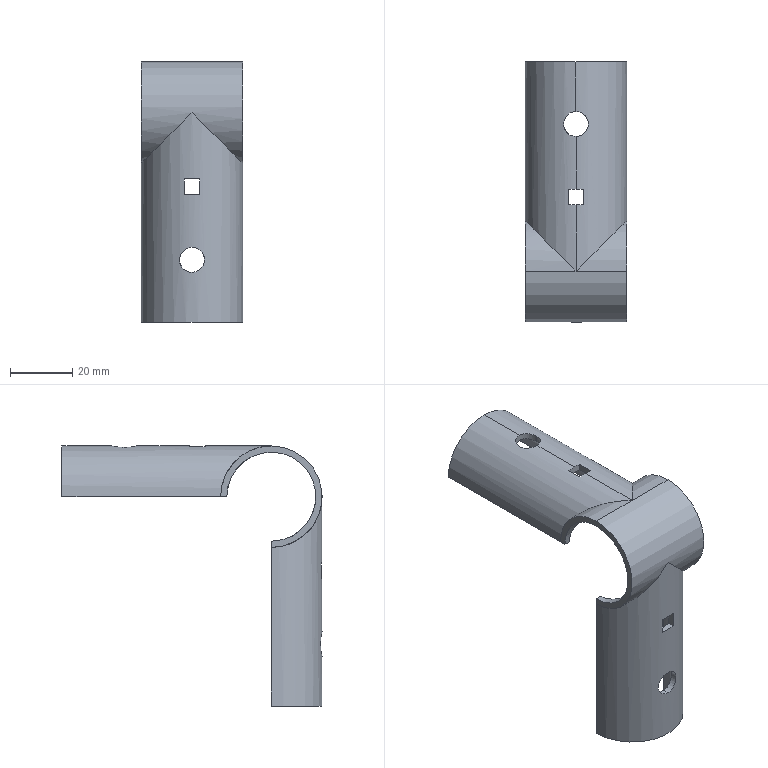Part | STEP file | F-C | 1 solid | 32 faces | box 32.6 x 83.6 x 83.6 mm | volume 13591 mm3 | cylinder 16 | plane 16 | commonest cylinder face diameters 28.6 x6 32.6 x6 8 x4